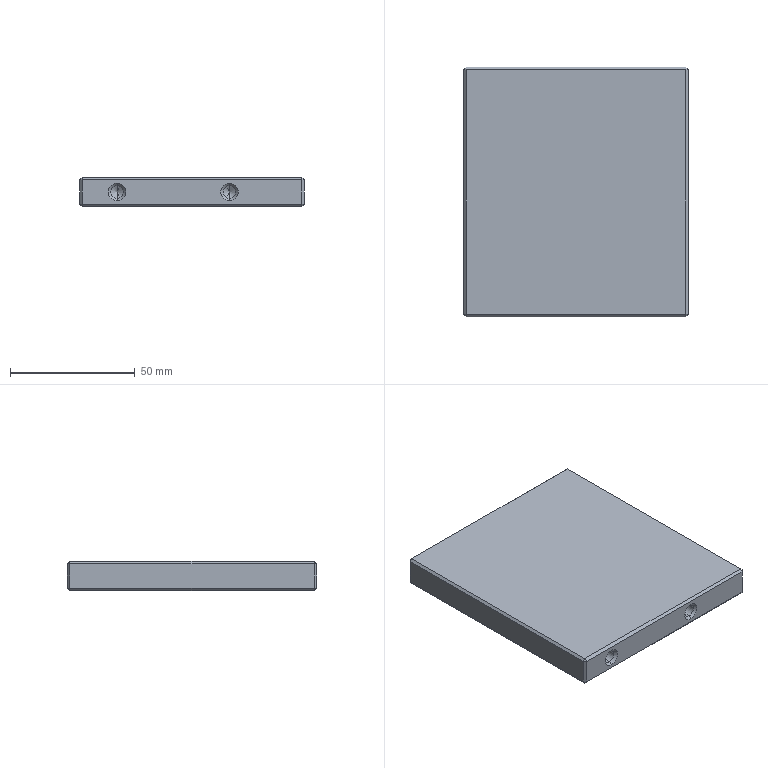Part | STEP file | 04-05 bending support plate | 1 solid | 55 faces | box 90 x 100 x 12 mm | volume 106188 mm3 | plane 27 | cone 18 | cylinder 10 | commonest cylinder face diameters 4.2 x4 5 x4 6 x2
STEP:
#1=CARTESIAN_POINT('',(0.,49.,3.));
#2=VERTEX_POINT('',#1);
#3=CARTESIAN_POINT('',(0.,49.,9.));
#4=VERTEX_POINT('',#3);
#5=CARTESIAN_POINT('',(0.,49.,6.));
#6=DIRECTION('',(0.,1.,0.));
#7=DIRECTION('',(0.,0.,-1.));
#8=AXIS2_PLACEMENT_3D('',#5,#6,#7);
#9=CIRCLE('',#8,3.);
#10=EDGE_CURVE('',#2,#4,#9,.T.);
#11=ORIENTED_EDGE('',*,*,#10,.F.);
#12=CARTESIAN_POINT('',(0.,50.,2.));
#13=VERTEX_POINT('',#12);
#14=CARTESIAN_POINT('',(0.,49.,3.));
#15=DIRECTION('',(0.,0.7071,-0.7071));
#16=VECTOR('',#15,1000.);
#17=LINE('',#14,#16);
#18=EDGE_CURVE('',#2,#13,#17,.T.);
#19=ORIENTED_EDGE('',*,*,#18,.T.);
#20=CARTESIAN_POINT('',(0.,50.,10.));
#21=VERTEX_POINT('',#20);
#22=CARTESIAN_POINT('',(0.,50.,6.));
#23=DIRECTION('',(0.,-1.,0.));
#24=DIRECTION('',(0.,0.,-1.));
#25=AXIS2_PLACEMENT_3D('',#22,#23,#24);
#26=CIRCLE('',#25,4.);
#27=EDGE_CURVE('',#21,#13,#26,.T.);
#28=ORIENTED_EDGE('',*,*,#27,.F.);
#29=CARTESIAN_POINT('',(0.,49.,9.));
#30=DIRECTION('',(0.,0.7071,0.7071));
#31=VECTOR('',#30,1000.);
#32=LINE('',#29,#31);
#33=EDGE_CURVE('',#4,#21,#32,.T.);
#34=ORIENTED_EDGE('',*,*,#33,.F.);
#35=EDGE_LOOP('',(#11,#19,#28,#34));
#36=FACE_OUTER_BOUND('',#35,.T.);
#37=CARTESIAN_POINT('',(0.,49.,6.));
#38=DIRECTION('',(0.,1.,0.));
#39=DIRECTION('',(0.,0.,1.));
#40=AXIS2_PLACEMENT_3D('',#37,#38,#39);
#41=CONICAL_SURFACE('',#40,3.,0.7854);
#42=ADVANCED_FACE('',(#36),#41,.F.);
#43=CARTESIAN_POINT('',(-30.,49.,3.9));
#44=VERTEX_POINT('',#43);
#45=CARTESIAN_POINT('',(-30.,49.,8.1));
#46=VERTEX_POINT('',#45);
#47=CARTESIAN_POINT('',(-30.,49.,6.));
#48=DIRECTION('',(0.,1.,0.));
#49=DIRECTION('',(0.,0.,-1.));
#50=AXIS2_PLACEMENT_3D('',#47,#48,#49);
#51=CIRCLE('',#50,2.1);
#52=EDGE_CURVE('',#44,#46,#51,.T.);
#53=ORIENTED_EDGE('',*,*,#52,.F.);
#54=CARTESIAN_POINT('',(-30.,50.,2.9));
#55=VERTEX_POINT('',#54);
#56=CARTESIAN_POINT('',(-30.,49.,3.9));
#57=DIRECTION('',(0.,0.7071,-0.7071));
#58=VECTOR('',#57,1000.);
#59=LINE('',#56,#58);
#60=EDGE_CURVE('',#44,#55,#59,.T.);
#61=ORIENTED_EDGE('',*,*,#60,.T.);
#62=CARTESIAN_POINT('',(-30.,50.,9.1));
#63=VERTEX_POINT('',#62);
#64=CARTESIAN_POINT('',(-30.,50.,6.));
#65=DIRECTION('',(0.,-1.,0.));
#66=DIRECTION('',(0.,0.,-1.));
#67=AXIS2_PLACEMENT_3D('',#64,#65,#66);
#68=CIRCLE('',#67,3.1);
#69=EDGE_CURVE('',#63,#55,#68,.T.);
#70=ORIENTED_EDGE('',*,*,#69,.F.);
#71=CARTESIAN_POINT('',(-30.,49.,8.1));
#72=DIRECTION('',(0.,0.7071,0.7071));
#73=VECTOR('',#72,1000.);
#74=LINE('',#71,#73);
#75=EDGE_CURVE('',#46,#63,#74,.T.);
#76=ORIENTED_EDGE('',*,*,#75,.F.);
#77=EDGE_LOOP('',(#53,#61,#70,#76));
#78=FACE_OUTER_BOUND('',#77,.T.);
#79=CARTESIAN_POINT('',(-30.,49.,6.));
#80=DIRECTION('',(0.,1.,0.));
#81=DIRECTION('',(0.,0.,1.));
#82=AXIS2_PLACEMENT_3D('',#79,#80,#81);
#83=CONICAL_SURFACE('',#82,2.1,0.7854);
#84=ADVANCED_FACE('',(#78),#83,.F.);
#85=CARTESIAN_POINT('',(30.,49.,3.9));
#86=VERTEX_POINT('',#85);
#87=CARTESIAN_POINT('',(30.,49.,8.1));
#88=VERTEX_POINT('',#87);
#89=CARTESIAN_POINT('',(30.,49.,6.));
#90=DIRECTION('',(0.,1.,0.));
#91=DIRECTION('',(0.,0.,-1.));
#92=AXIS2_PLACEMENT_3D('',#89,#90,#91);
#93=CIRCLE('',#92,2.1);
#94=EDGE_CURVE('',#86,#88,#93,.T.);
#95=ORIENTED_EDGE('',*,*,#94,.F.);
#96=CARTESIAN_POINT('',(30.,50.,2.9));
#97=VERTEX_POINT('',#96);
#98=CARTESIAN_POINT('',(30.,49.,3.9));
#99=DIRECTION('',(0.,0.7071,-0.7071));
#100=VECTOR('',#99,1000.);
#101=LINE('',#98,#100);
#102=EDGE_CURVE('',#86,#97,#101,.T.);
#103=ORIENTED_EDGE('',*,*,#102,.T.);
#104=CARTESIAN_POINT('',(30.,50.,9.1));
#105=VERTEX_POINT('',#104);
#106=CARTESIAN_POINT('',(30.,50.,6.));
#107=DIRECTION('',(0.,-1.,0.));
#108=DIRECTION('',(0.,0.,-1.));
#109=AXIS2_PLACEMENT_3D('',#106,#107,#108);
#110=CIRCLE('',#109,3.1);
#111=EDGE_CURVE('',#105,#97,#110,.T.);
#112=ORIENTED_EDGE('',*,*,#111,.F.);
#113=CARTESIAN_POINT('',(30.,49.,8.1));
#114=DIRECTION('',(0.,0.7071,0.7071));
#115=VECTOR('',#114,1000.);
#116=LINE('',#113,#115);
#117=EDGE_CURVE('',#88,#105,#116,.T.);
#118=ORIENTED_EDGE('',*,*,#117,.F.);
#119=EDGE_LOOP('',(#95,#103,#112,#118));
#120=FACE_OUTER_BOUND('',#119,.T.);
#121=CARTESIAN_POINT('',(30.,49.,6.));
#122=DIRECTION('',(0.,1.,0.));
#123=DIRECTION('',(0.,0.,1.));
#124=AXIS2_PLACEMENT_3D('',#121,#122,#123);
#125=CONICAL_SURFACE('',#124,2.1,0.7854);
#126=ADVANCED_FACE('',(#120),#125,.F.);
#127=CARTESIAN_POINT('',(-30.,-49.,8.5));
#128=VERTEX_POINT('',#127);
#129=CARTESIAN_POINT('',(-30.,-49.,3.5));
#130=VERTEX_POINT('',#129);
#131=CARTESIAN_POINT('',(-30.,-49.,6.));
#132=DIRECTION('',(0.,-1.,0.));
#133=DIRECTION('',(0.,0.,1.));
#134=AXIS2_PLACEMENT_3D('',#131,#132,#133);
#135=CIRCLE('',#134,2.5);
#136=EDGE_CURVE('',#128,#130,#135,.T.);
#137=ORIENTED_EDGE('',*,*,#136,.F.);
#138=CARTESIAN_POINT('',(-30.,-50.,9.5));
#139=VERTEX_POINT('',#138);
#140=CARTESIAN_POINT('',(-30.,-49.,8.5));
#141=DIRECTION('',(0.,-0.7071,0.7071));
#142=VECTOR('',#141,1000.);
#143=LINE('',#140,#142);
#144=EDGE_CURVE('',#128,#139,#143,.T.);
#145=ORIENTED_EDGE('',*,*,#144,.T.);
#146=CARTESIAN_POINT('',(-30.,-50.,2.5));
#147=VERTEX_POINT('',#146);
#148=CARTESIAN_POINT('',(-30.,-50.,6.));
#149=DIRECTION('',(0.,1.,0.));
#150=DIRECTION('',(0.,0.,1.));
#151=AXIS2_PLACEMENT_3D('',#148,#149,#150);
#152=CIRCLE('',#151,3.5);
#153=EDGE_CURVE('',#147,#139,#152,.T.);
#154=ORIENTED_EDGE('',*,*,#153,.F.);
#155=CARTESIAN_POINT('',(-30.,-49.,3.5));
#156=DIRECTION('',(0.,-0.7071,-0.7071));
#157=VECTOR('',#156,1000.);
#158=LINE('',#155,#157);
#159=EDGE_CURVE('',#130,#147,#158,.T.);
#160=ORIENTED_EDGE('',*,*,#159,.F.);
#161=EDGE_LOOP('',(#137,#145,#154,#160));
#162=FACE_OUTER_BOUND('',#161,.T.);
#163=CARTESIAN_POINT('',(-30.,-49.,6.));
#164=DIRECTION('',(0.,-1.,0.));
#165=DIRECTION('',(0.,0.,-1.));
#166=AXIS2_PLACEMENT_3D('',#163,#164,#165);
#167=CONICAL_SURFACE('',#166,2.5,0.7854);
#168=ADVANCED_FACE('',(#162),#167,.F.);
#169=CARTESIAN_POINT('',(15.,-49.,8.5));
#170=VERTEX_POINT('',#169);
#171=CARTESIAN_POINT('',(15.,-49.,3.5));
#172=VERTEX_POINT('',#171);
#173=CARTESIAN_POINT('',(15.,-49.,6.));
#174=DIRECTION('',(0.,-1.,0.));
#175=DIRECTION('',(0.,0.,1.));
#176=AXIS2_PLACEMENT_3D('',#173,#174,#175);
#177=CIRCLE('',#176,2.5);
#178=EDGE_CURVE('',#170,#172,#177,.T.);
#179=ORIENTED_EDGE('',*,*,#178,.F.);
#180=CARTESIAN_POINT('',(15.,-50.,9.5));
#181=VERTEX_POINT('',#180);
#182=CARTESIAN_POINT('',(15.,-49.,8.5));
#183=DIRECTION('',(0.,-0.7071,0.7071));
#184=VECTOR('',#183,1000.);
#185=LINE('',#182,#184);
#186=EDGE_CURVE('',#170,#181,#185,.T.);
#187=ORIENTED_EDGE('',*,*,#186,.T.);
#188=CARTESIAN_POINT('',(15.,-50.,2.5));
#189=VERTEX_POINT('',#188);
#190=CARTESIAN_POINT('',(15.,-50.,6.));
#191=DIRECTION('',(0.,1.,0.));
#192=DIRECTION('',(0.,0.,1.));
#193=AXIS2_PLACEMENT_3D('',#190,#191,#192);
#194=CIRCLE('',#193,3.5);
#195=EDGE_CURVE('',#189,#181,#194,.T.);
#196=ORIENTED_EDGE('',*,*,#195,.F.);
#197=CARTESIAN_POINT('',(15.,-49.,3.5));
#198=DIRECTION('',(0.,-0.7071,-0.7071));
#199=VECTOR('',#198,1000.);
#200=LINE('',#197,#199);
#201=EDGE_CURVE('',#172,#189,#200,.T.);
#202=ORIENTED_EDGE('',*,*,#201,.F.);
#203=EDGE_LOOP('',(#179,#187,#196,#202));
#204=FACE_OUTER_BOUND('',#203,.T.);
#205=CARTESIAN_POINT('',(15.,-49.,6.));
#206=DIRECTION('',(0.,-1.,0.));
#207=DIRECTION('',(0.,0.,-1.));
#208=AXIS2_PLACEMENT_3D('',#205,#206,#207);
#209=CONICAL_SURFACE('',#208,2.5,0.7854);
#210=ADVANCED_FACE('',(#204),#209,.F.);
#211=CARTESIAN_POINT('',(0.,40.,3.));
#212=VERTEX_POINT('',#211);
#213=CARTESIAN_POINT('',(0.,40.,9.));
#214=VERTEX_POINT('',#213);
#215=CARTESIAN_POINT('',(0.,40.,6.));
#216=DIRECTION('',(0.,1.,0.));
#217=DIRECTION('',(0.,0.,1.));
#218=AXIS2_PLACEMENT_3D('',#215,#216,#217);
#219=CIRCLE('',#218,3.);
#220=EDGE_CURVE('',#212,#214,#219,.T.);
#221=ORIENTED_EDGE('',*,*,#220,.F.);
#222=CARTESIAN_POINT('',(0.,40.,3.));
#223=DIRECTION('',(0.,1.,0.));
#224=VECTOR('',#223,1000.);
#225=LINE('',#222,#224);
#226=EDGE_CURVE('',#212,#2,#225,.T.);
#227=ORIENTED_EDGE('',*,*,#226,.T.);
#228=ORIENTED_EDGE('',*,*,#10,.T.);
#229=CARTESIAN_POINT('',(0.,40.,9.));
#230=DIRECTION('',(0.,1.,0.));
#231=VECTOR('',#230,1000.);
#232=LINE('',#229,#231);
#233=EDGE_CURVE('',#214,#4,#232,.T.);
#234=ORIENTED_EDGE('',*,*,#233,.F.);
#235=EDGE_LOOP('',(#221,#227,#228,#234));
#236=FACE_OUTER_BOUND('',#235,.T.);
#237=CARTESIAN_POINT('',(0.,40.,6.));
#238=DIRECTION('',(0.,1.,0.));
#239=DIRECTION('',(0.,0.,1.));
#240=AXIS2_PLACEMENT_3D('',#237,#238,#239);
#241=CYLINDRICAL_SURFACE('',#240,3.);
#242=ADVANCED_FACE('',(#236),#241,.F.);
#243=CARTESIAN_POINT('',(-30.,36.,3.9));
#244=VERTEX_POINT('',#243);
#245=CARTESIAN_POINT('',(-30.,36.,8.1));
#246=VERTEX_POINT('',#245);
#247=CARTESIAN_POINT('',(-30.,36.,6.));
#248=DIRECTION('',(0.,1.,0.));
#249=DIRECTION('',(0.,0.,1.));
#250=AXIS2_PLACEMENT_3D('',#247,#248,#249);
#251=CIRCLE('',#250,2.1);
#252=EDGE_CURVE('',#244,#246,#251,.T.);
#253=ORIENTED_EDGE('',*,*,#252,.F.);
#254=CARTESIAN_POINT('',(-30.,50.,3.9));
#255=DIRECTION('',(0.,1.,0.));
#256=VECTOR('',#255,1000.);
#257=LINE('',#254,#256);
#258=EDGE_CURVE('',#244,#44,#257,.T.);
#259=ORIENTED_EDGE('',*,*,#258,.T.);
#260=ORIENTED_EDGE('',*,*,#52,.T.);
#261=CARTESIAN_POINT('',(-30.,50.,8.1));
#262=DIRECTION('',(0.,1.,0.));
#263=VECTOR('',#262,1000.);
#264=LINE('',#261,#263);
#265=EDGE_CURVE('',#246,#46,#264,.T.);
#266=ORIENTED_EDGE('',*,*,#265,.F.);
#267=EDGE_LOOP('',(#253,#259,#260,#266));
#268=FACE_OUTER_BOUND('',#267,.T.);
#269=CARTESIAN_POINT('',(-30.,50.,6.));
#270=DIRECTION('',(0.,1.,0.));
#271=DIRECTION('',(0.,0.,1.));
#272=AXIS2_PLACEMENT_3D('',#269,#270,#271);
#273=CYLINDRICAL_SURFACE('',#272,2.1);
#274=ADVANCED_FACE('',(#268),#273,.F.);
#275=CARTESIAN_POINT('',(-30.,34.738,6.));
#276=VERTEX_POINT('',#275);
#277=CARTESIAN_POINT('',(-30.,36.,8.1));
#278=DIRECTION('',(0.,0.515,0.8572));
#279=VECTOR('',#278,1000.);
#280=LINE('',#277,#279);
#281=EDGE_CURVE('',#276,#246,#280,.T.);
#282=ORIENTED_EDGE('',*,*,#281,.F.);
#283=CARTESIAN_POINT('',(-30.,36.,3.9));
#284=DIRECTION('',(0.,0.515,-0.8572));
#285=VECTOR('',#284,1000.);
#286=LINE('',#283,#285);
#287=EDGE_CURVE('',#276,#244,#286,.T.);
#288=ORIENTED_EDGE('',*,*,#287,.T.);
#289=ORIENTED_EDGE('',*,*,#252,.T.);
#290=EDGE_LOOP('',(#282,#288,#289));
#291=FACE_OUTER_BOUND('',#290,.T.);
#292=CARTESIAN_POINT('',(-30.,36.,6.));
#293=DIRECTION('',(0.,1.,0.));
#294=DIRECTION('',(0.,0.,1.));
#295=AXIS2_PLACEMENT_3D('',#292,#293,#294);
#296=CONICAL_SURFACE('',#295,2.1,1.03);
#297=ADVANCED_FACE('',(#291),#296,.F.);
#298=CARTESIAN_POINT('',(30.,36.,3.9));
#299=VERTEX_POINT('',#298);
#300=CARTESIAN_POINT('',(30.,36.,8.1));
#301=VERTEX_POINT('',#300);
#302=CARTESIAN_POINT('',(30.,36.,6.));
#303=DIRECTION('',(0.,1.,0.));
#304=DIRECTION('',(0.,0.,1.));
#305=AXIS2_PLACEMENT_3D('',#302,#303,#304);
#306=CIRCLE('',#305,2.1);
#307=EDGE_CURVE('',#299,#301,#306,.T.);
#308=ORIENTED_EDGE('',*,*,#307,.F.);
#309=CARTESIAN_POINT('',(30.,50.,3.9));
#310=DIRECTION('',(0.,1.,0.));
#311=VECTOR('',#310,1000.);
#312=LINE('',#309,#311);
#313=EDGE_CURVE('',#299,#86,#312,.T.);
#314=ORIENTED_EDGE('',*,*,#313,.T.);
#315=ORIENTED_EDGE('',*,*,#94,.T.);
#316=CARTESIAN_POINT('',(30.,50.,8.1));
#317=DIRECTION('',(0.,1.,0.));
#318=VECTOR('',#317,1000.);
#319=LINE('',#316,#318);
#320=EDGE_CURVE('',#301,#88,#319,.T.);
#321=ORIENTED_EDGE('',*,*,#320,.F.);
#322=EDGE_LOOP('',(#308,#314,#315,#321));
#323=FACE_OUTER_BOUND('',#322,.T.);
#324=CARTESIAN_POINT('',(30.,50.,6.));
#325=DIRECTION('',(0.,1.,0.));
#326=DIRECTION('',(0.,0.,1.));
#327=AXIS2_PLACEMENT_3D('',#324,#325,#326);
#328=CYLINDRICAL_SURFACE('',#327,2.1);
#329=ADVANCED_FACE('',(#323),#328,.F.);
#330=CARTESIAN_POINT('',(30.,34.738,6.));
#331=VERTEX_POINT('',#330);
#332=CARTESIAN_POINT('',(30.,36.,8.1));
#333=DIRECTION('',(0.,0.515,0.8572));
#334=VECTOR('',#333,1000.);
#335=LINE('',#332,#334);
#336=EDGE_CURVE('',#331,#301,#335,.T.);
#337=ORIENTED_EDGE('',*,*,#336,.F.);
#338=CARTESIAN_POINT('',(30.,36.,3.9));
#339=DIRECTION('',(0.,0.515,-0.8572));
#340=VECTOR('',#339,1000.);
#341=LINE('',#338,#340);
#342=EDGE_CURVE('',#331,#299,#341,.T.);
#343=ORIENTED_EDGE('',*,*,#342,.T.);
#344=ORIENTED_EDGE('',*,*,#307,.T.);
#345=EDGE_LOOP('',(#337,#343,#344));
#346=FACE_OUTER_BOUND('',#345,.T.);
#347=CARTESIAN_POINT('',(30.,36.,6.));
#348=DIRECTION('',(0.,1.,0.));
#349=DIRECTION('',(0.,0.,1.));
#350=AXIS2_PLACEMENT_3D('',#347,#348,#349);
#351=CONICAL_SURFACE('',#350,2.1,1.03);
#352=ADVANCED_FACE('',(#346),#351,.F.);
#353=CARTESIAN_POINT('',(-30.,-33.,8.5));
#354=VERTEX_POINT('',#353);
#355=CARTESIAN_POINT('',(-30.,-33.,3.5));
#356=VERTEX_POINT('',#355);
#357=CARTESIAN_POINT('',(-30.,-33.,6.));
#358=DIRECTION('',(0.,-1.,0.));
#359=DIRECTION('',(0.,0.,-1.));
#360=AXIS2_PLACEMENT_3D('',#357,#358,#359);
#361=CIRCLE('',#360,2.5);
#362=EDGE_CURVE('',#354,#356,#361,.T.);
#363=ORIENTED_EDGE('',*,*,#362,.F.);
#364=CARTESIAN_POINT('',(-30.,-50.,8.5));
#365=DIRECTION('',(0.,-1.,0.));
#366=VECTOR('',#365,1000.);
#367=LINE('',#364,#366);
#368=EDGE_CURVE('',#354,#128,#367,.T.);
#369=ORIENTED_EDGE('',*,*,#368,.T.);
#370=ORIENTED_EDGE('',*,*,#136,.T.);
#371=CARTESIAN_POINT('',(-30.,-50.,3.5));
#372=DIRECTION('',(0.,-1.,0.));
#373=VECTOR('',#372,1000.);
#374=LINE('',#371,#373);
#375=EDGE_CURVE('',#356,#130,#374,.T.);
#376=ORIENTED_EDGE('',*,*,#375,.F.);
#377=EDGE_LOOP('',(#363,#369,#370,#376));
#378=FACE_OUTER_BOUND('',#377,.T.);
#379=CARTESIAN_POINT('',(-30.,-50.,6.));
#380=DIRECTION('',(0.,-1.,0.));
#381=DIRECTION('',(0.,0.,-1.));
#382=AXIS2_PLACEMENT_3D('',#379,#380,#381);
#383=CYLINDRICAL_SURFACE('',#382,2.5);
#384=ADVANCED_FACE('',(#378),#383,.F.);
#385=CARTESIAN_POINT('',(-30.,-31.498,6.));
#386=VERTEX_POINT('',#385);
#387=CARTESIAN_POINT('',(-30.,-33.,3.5));
#388=DIRECTION('',(0.,-0.515,-0.8572));
#389=VECTOR('',#388,1000.);
#390=LINE('',#387,#389);
#391=EDGE_CURVE('',#386,#356,#390,.T.);
#392=ORIENTED_EDGE('',*,*,#391,.F.);
#393=CARTESIAN_POINT('',(-30.,-33.,8.5));
#394=DIRECTION('',(0.,-0.515,0.8572));
#395=VECTOR('',#394,1000.);
#396=LINE('',#393,#395);
#397=EDGE_CURVE('',#386,#354,#396,.T.);
#398=ORIENTED_EDGE('',*,*,#397,.T.);
#399=ORIENTED_EDGE('',*,*,#362,.T.);
#400=EDGE_LOOP('',(#392,#398,#399));
#401=FACE_OUTER_BOUND('',#400,.T.);
#402=CARTESIAN_POINT('',(-30.,-33.,6.));
#403=DIRECTION('',(0.,-1.,0.));
#404=DIRECTION('',(0.,0.,-1.));
#405=AXIS2_PLACEMENT_3D('',#402,#403,#404);
#406=CONICAL_SURFACE('',#405,2.5,1.03);
#407=ADVANCED_FACE('',(#401),#406,.F.);
#408=CARTESIAN_POINT('',(15.,-33.,8.5));
#409=VERTEX_POINT('',#408);
#410=CARTESIAN_POINT('',(15.,-33.,3.5));
#411=VERTEX_POINT('',#410);
#412=CARTESIAN_POINT('',(15.,-33.,6.));
#413=DIRECTION('',(0.,-1.,0.));
#414=DIRECTION('',(0.,0.,-1.));
#415=AXIS2_PLACEMENT_3D('',#412,#413,#414);
#416=CIRCLE('',#415,2.5);
#417=EDGE_CURVE('',#409,#411,#416,.T.);
#418=ORIENTED_EDGE('',*,*,#417,.F.);
#419=CARTESIAN_POINT('',(15.,-50.,8.5));
#420=DIRECTION('',(0.,-1.,0.));
#421=VECTOR('',#420,1000.);
#422=LINE('',#419,#421);
#423=EDGE_CURVE('',#409,#170,#422,.T.);
#424=ORIENTED_EDGE('',*,*,#423,.T.);
#425=ORIENTED_EDGE('',*,*,#178,.T.);
#426=CARTESIAN_POINT('',(15.,-50.,3.5));
#427=DIRECTION('',(0.,-1.,0.));
#428=VECTOR('',#427,1000.);
#429=LINE('',#426,#428);
#430=EDGE_CURVE('',#411,#172,#429,.T.);
#431=ORIENTED_EDGE('',*,*,#430,.F.);
#432=EDGE_LOOP('',(#418,#424,#425,#431));
#433=FACE_OUTER_BOUND('',#432,.T.);
#434=CARTESIAN_POINT('',(15.,-50.,6.));
#435=DIRECTION('',(0.,-1.,0.));
#436=DIRECTION('',(0.,0.,-1.));
#437=AXIS2_PLACEMENT_3D('',#434,#435,#436);
#438=CYLINDRICAL_SURFACE('',#437,2.5);
#439=ADVANCED_FACE('',(#433),#438,.F.);
#440=CARTESIAN_POINT('',(15.,-31.498,6.));
#441=VERTEX_POINT('',#440);
#442=CARTESIAN_POINT('',(15.,-33.,3.5));
#443=DIRECTION('',(0.,-0.515,-0.8572));
#444=VECTOR('',#443,1000.);
#445=LINE('',#442,#444);
#446=EDGE_CURVE('',#441,#411,#445,.T.);
#447=ORIENTED_EDGE('',*,*,#446,.F.);
#448=CARTESIAN_POINT('',(15.,-33.,8.5));
#449=DIRECTION('',(0.,-0.515,0.8572));
#450=VECTOR('',#449,1000.);
#451=LINE('',#448,#450);
#452=EDGE_CURVE('',#441,#409,#451,.T.);
#453=ORIENTED_EDGE('',*,*,#452,.T.);
#454=ORIENTED_EDGE('',*,*,#417,.T.);
#455=EDGE_LOOP('',(#447,#453,#454));
#456=FACE_OUTER_BOUND('',#455,.T.);
#457=CARTESIAN_POINT('',(15.,-33.,6.));
#458=DIRECTION('',(0.,-1.,0.));
#459=DIRECTION('',(0.,0.,-1.));
#460=AXIS2_PLACEMENT_3D('',#457,#458,#459);
#461=CONICAL_SURFACE('',#460,2.5,1.03);
#462=ADVANCED_FACE('',(#456),#461,.F.);
#463=CARTESIAN_POINT('',(45.,-49.,11.));
#464=VERTEX_POINT('',#463);
#465=CARTESIAN_POINT('',(45.,-49.,1.));
#466=VERTEX_POINT('',#465);
#467=CARTESIAN_POINT('',(45.,-49.,12.));
#468=DIRECTION('',(0.,0.,-1.));
#469=VECTOR('',#468,1000.);
#470=LINE('',#467,#469);
#471=EDGE_CURVE('',#464,#466,#470,.T.);
#472=ORIENTED_EDGE('',*,*,#471,.T.);
#473=CARTESIAN_POINT('',(45.,49.,1.));
#474=VERTEX_POINT('',#473);
#475=CARTESIAN_POINT('',(45.,50.,1.));
#476=DIRECTION('',(0.,1.,0.));
#477=VECTOR('',#476,1000.);
#478=LINE('',#475,#477);
#479=EDGE_CURVE('',#466,#474,#478,.T.);
#480=ORIENTED_EDGE('',*,*,#479,.T.);
#481=CARTESIAN_POINT('',(45.,49.,11.));
#482=VERTEX_POINT('',#481);
#483=CARTESIAN_POINT('',(45.,49.,12.));
#484=DIRECTION('',(0.,0.,1.));
#485=VECTOR('',#484,1000.);
#486=LINE('',#483,#485);
#487=EDGE_CURVE('',#474,#482,#486,.T.);
#488=ORIENTED_EDGE('',*,*,#487,.T.);
#489=CARTESIAN_POINT('',(45.,-50.,11.));
#490=DIRECTION('',(0.,-1.,0.));
#491=VECTOR('',#490,1000.);
#492=LINE('',#489,#491);
#493=EDGE_CURVE('',#482,#464,#492,.T.);
#494=ORIENTED_EDGE('',*,*,#493,.T.);
#495=EDGE_LOOP('',(#472,#480,#488,#494));
#496=FACE_OUTER_BOUND('',#495,.T.);
#497=CARTESIAN_POINT('',(45.,50.,12.));
#498=DIRECTION('',(-1.,0.,0.));
#499=DIRECTION('',(0.,-1.,0.));
#500=AXIS2_PLACEMENT_3D('',#497,#498,#499);
#501=PLANE('',#500);
#502=ADVANCED_FACE('',(#496),#501,.F.);
#503=ORIENTED_EDGE('',*,*,#111,.T.);
#504=CARTESIAN_POINT('',(30.,50.,6.));
#505=DIRECTION('',(0.,-1.,0.));
#506=DIRECTION('',(0.,0.,-1.));
#507=AXIS2_PLACEMENT_3D('',#504,#505,#506);
#508=CIRCLE('',#507,3.1);
#509=EDGE_CURVE('',#97,#105,#508,.T.);
#510=ORIENTED_EDGE('',*,*,#509,.T.);
#511=EDGE_LOOP('',(#503,#510));
#512=FACE_BOUND('',#511,.T.);
#513=ORIENTED_EDGE('',*,*,#69,.T.);
#514=CARTESIAN_POINT('',(-30.,50.,6.));
#515=DIRECTION('',(0.,-1.,0.));
#516=DIRECTION('',(0.,0.,-1.));
#517=AXIS2_PLACEMENT_3D('',#514,#515,#516);
#518=CIRCLE('',#517,3.1);
#519=EDGE_CURVE('',#55,#63,#518,.T.);
#520=ORIENTED_EDGE('',*,*,#519,.T.);
#521=EDGE_LOOP('',(#513,#520));
#522=FACE_BOUND('',#521,.T.);
#523=ORIENTED_EDGE('',*,*,#27,.T.);
#524=CARTESIAN_POINT('',(0.,50.,6.));
#525=DIRECTION('',(0.,-1.,0.));
#526=DIRECTION('',(0.,0.,-1.));
#527=AXIS2_PLACEMENT_3D('',#524,#525,#526);
#528=CIRCLE('',#527,4.);
#529=EDGE_CURVE('',#13,#21,#528,.T.);
#530=ORIENTED_EDGE('',*,*,#529,.T.);
#531=EDGE_LOOP('',(#523,#530));
#532=FACE_BOUND('',#531,.T.);
#533=CARTESIAN_POINT('',(44.,50.,11.));
#534=VERTEX_POINT('',#533);
#535=CARTESIAN_POINT('',(44.,50.,1.));
#536=VERTEX_POINT('',#535);
#537=CARTESIAN_POINT('',(44.,50.,12.));
#538=DIRECTION('',(0.,0.,-1.));
#539=VECTOR('',#538,1000.);
#540=LINE('',#537,#539);
#541=EDGE_CURVE('',#534,#536,#540,.T.);
#542=ORIENTED_EDGE('',*,*,#541,.T.);
#543=CARTESIAN_POINT('',(-44.,50.,1.));
#544=VERTEX_POINT('',#543);
#545=CARTESIAN_POINT('',(-45.,50.,1.));
#546=DIRECTION('',(-1.,0.,0.));
#547=VECTOR('',#546,1000.);
#548=LINE('',#545,#547);
#549=EDGE_CURVE('',#536,#544,#548,.T.);
#550=ORIENTED_EDGE('',*,*,#549,.T.);
#551=CARTESIAN_POINT('',(-44.,50.,11.));
#552=VERTEX_POINT('',#551);
#553=CARTESIAN_POINT('',(-44.,50.,12.));
#554=DIRECTION('',(0.,0.,1.));
#555=VECTOR('',#554,1000.);
#556=LINE('',#553,#555);
#557=EDGE_CURVE('',#544,#552,#556,.T.);
#558=ORIENTED_EDGE('',*,*,#557,.T.);
#559=CARTESIAN_POINT('',(45.,50.,11.));
#560=DIRECTION('',(1.,0.,0.));
#561=VECTOR('',#560,1000.);
#562=LINE('',#559,#561);
#563=EDGE_CURVE('',#552,#534,#562,.T.);
#564=ORIENTED_EDGE('',*,*,#563,.T.);
#565=EDGE_LOOP('',(#542,#550,#558,#564));
#566=FACE_OUTER_BOUND('',#565,.T.);
#567=CARTESIAN_POINT('',(-45.,50.,12.));
#568=DIRECTION('',(0.,-1.,0.));
#569=DIRECTION('',(0.,0.,-1.));
#570=AXIS2_PLACEMENT_3D('',#567,#568,#569);
#571=PLANE('',#570);
#572=ADVANCED_FACE('',(#512,#522,#532,#566),#571,.F.);
#573=CARTESIAN_POINT('',(-45.,-49.,11.));
#574=VERTEX_POINT('',#573);
#575=CARTESIAN_POINT('',(-45.,49.,11.));
#576=VERTEX_POINT('',#575);
#577=CARTESIAN_POINT('',(-45.,50.,11.));
#578=DIRECTION('',(0.,1.,0.));
#579=VECTOR('',#578,1000.);
#580=LINE('',#577,#579);
#581=EDGE_CURVE('',#574,#576,#580,.T.);
#582=ORIENTED_EDGE('',*,*,#581,.T.);
#583=CARTESIAN_POINT('',(-45.,49.,1.));
#584=VERTEX_POINT('',#583);
#585=CARTESIAN_POINT('',(-45.,49.,12.));
#586=DIRECTION('',(0.,0.,-1.));
#587=VECTOR('',#586,1000.);
#588=LINE('',#585,#587);
#589=EDGE_CURVE('',#576,#584,#588,.T.);
#590=ORIENTED_EDGE('',*,*,#589,.T.);
#591=CARTESIAN_POINT('',(-45.,-49.,1.));
#592=VERTEX_POINT('',#591);
#593=CARTESIAN_POINT('',(-45.,50.,1.));
#594=DIRECTION('',(0.,-1.,0.));
#595=VECTOR('',#594,1000.);
#596=LINE('',#593,#595);
#597=EDGE_CURVE('',#584,#592,#596,.T.);
#598=ORIENTED_EDGE('',*,*,#597,.T.);
#599=CARTESIAN_POINT('',(-45.,-49.,12.));
#600=DIRECTION('',(0.,0.,1.));
#601=VECTOR('',#600,1000.);
#602=LINE('',#599,#601);
#603=EDGE_CURVE('',#592,#574,#602,.T.);
#604=ORIENTED_EDGE('',*,*,#603,.T.);
#605=EDGE_LOOP('',(#582,#590,#598,#604));
#606=FACE_OUTER_BOUND('',#605,.T.);
#607=CARTESIAN_POINT('',(-45.,50.,12.));
#608=DIRECTION('',(1.,0.,0.));
#609=DIRECTION('',(0.,1.,0.));
#610=AXIS2_PLACEMENT_3D('',#607,#608,#609);
#611=PLANE('',#610);
#612=ADVANCED_FACE('',(#606),#611,.F.);
#613=ORIENTED_EDGE('',*,*,#195,.T.);
#614=CARTESIAN_POINT('',(15.,-50.,6.));
#615=DIRECTION('',(0.,1.,0.));
#616=DIRECTION('',(0.,0.,1.));
#617=AXIS2_PLACEMENT_3D('',#614,#615,#616);
#618=CIRCLE('',#617,3.5);
#619=EDGE_CURVE('',#181,#189,#618,.T.);
#620=ORIENTED_EDGE('',*,*,#619,.T.);
#621=EDGE_LOOP('',(#613,#620));
#622=FACE_BOUND('',#621,.T.);
#623=ORIENTED_EDGE('',*,*,#153,.T.);
#624=CARTESIAN_POINT('',(-30.,-50.,6.));
#625=DIRECTION('',(0.,1.,0.));
#626=DIRECTION('',(0.,0.,1.));
#627=AXIS2_PLACEMENT_3D('',#624,#625,#626);
#628=CIRCLE('',#627,3.5);
#629=EDGE_CURVE('',#139,#147,#628,.T.);
#630=ORIENTED_EDGE('',*,*,#629,.T.);
#631=EDGE_LOOP('',(#623,#630));
#632=FACE_BOUND('',#631,.T.);
#633=CARTESIAN_POINT('',(-44.,-50.,1.));
#634=VERTEX_POINT('',#633);
#635=CARTESIAN_POINT('',(44.,-50.,1.));
#636=VERTEX_POINT('',#635);
#637=CARTESIAN_POINT('',(-45.,-50.,1.));
#638=DIRECTION('',(1.,0.,0.));
#639=VECTOR('',#638,1000.);
#640=LINE('',#637,#639);
#641=EDGE_CURVE('',#634,#636,#640,.T.);
#642=ORIENTED_EDGE('',*,*,#641,.T.);
#643=CARTESIAN_POINT('',(44.,-50.,11.));
#644=VERTEX_POINT('',#643);
#645=CARTESIAN_POINT('',(44.,-50.,12.));
#646=DIRECTION('',(0.,0.,1.));
#647=VECTOR('',#646,1000.);
#648=LINE('',#645,#647);
#649=EDGE_CURVE('',#636,#644,#648,.T.);
#650=ORIENTED_EDGE('',*,*,#649,.T.);
#651=CARTESIAN_POINT('',(-44.,-50.,11.));
#652=VERTEX_POINT('',#651);
#653=CARTESIAN_POINT('',(-45.,-50.,11.));
#654=DIRECTION('',(-1.,0.,0.));
#655=VECTOR('',#654,1000.);
#656=LINE('',#653,#655);
#657=EDGE_CURVE('',#644,#652,#656,.T.);
#658=ORIENTED_EDGE('',*,*,#657,.T.);
#659=CARTESIAN_POINT('',(-44.,-50.,12.));
#660=DIRECTION('',(0.,0.,-1.));
#661=VECTOR('',#660,1000.);
#662=LINE('',#659,#661);
#663=EDGE_CURVE('',#652,#634,#662,.T.);
#664=ORIENTED_EDGE('',*,*,#663,.T.);
#665=EDGE_LOOP('',(#642,#650,#658,#664));
#666=FACE_OUTER_BOUND('',#665,.T.);
#667=CARTESIAN_POINT('',(-45.,-50.,12.));
#668=DIRECTION('',(0.,1.,0.));
#669=DIRECTION('',(0.,0.,1.));
#670=AXIS2_PLACEMENT_3D('',#667,#668,#669);
#671=PLANE('',#670);
#672=ADVANCED_FACE('',(#622,#632,#666),#671,.F.);
#673=CARTESIAN_POINT('',(-44.,49.,12.));
#674=VERTEX_POINT('',#673);
#675=CARTESIAN_POINT('',(-44.,-49.,12.));
#676=VERTEX_POINT('',#675);
#677=CARTESIAN_POINT('',(-44.,-50.,12.));
#678=DIRECTION('',(0.,-1.,0.));
#679=VECTOR('',#678,1000.);
#680=LINE('',#677,#679);
#681=EDGE_CURVE('',#674,#676,#680,.T.);
#682=ORIENTED_EDGE('',*,*,#681,.T.);
#683=CARTESIAN_POINT('',(44.,-49.,12.));
#684=VERTEX_POINT('',#683);
#685=CARTESIAN_POINT('',(45.,-49.,12.));
#686=DIRECTION('',(1.,0.,0.));
#687=VECTOR('',#686,1000.);
#688=LINE('',#685,#687);
#689=EDGE_CURVE('',#676,#684,#688,.T.);
#690=ORIENTED_EDGE('',*,*,#689,.T.);
#691=CARTESIAN_POINT('',(44.,49.,12.));
#692=VERTEX_POINT('',#691);
#693=CARTESIAN_POINT('',(44.,50.,12.));
#694=DIRECTION('',(0.,1.,0.));
#695=VECTOR('',#694,1000.);
#696=LINE('',#693,#695);
#697=EDGE_CURVE('',#684,#692,#696,.T.);
#698=ORIENTED_EDGE('',*,*,#697,.T.);
#699=CARTESIAN_POINT('',(-45.,49.,12.));
#700=DIRECTION('',(-1.,0.,0.));
#701=VECTOR('',#700,1000.);
#702=LINE('',#699,#701);
#703=EDGE_CURVE('',#692,#674,#702,.T.);
#704=ORIENTED_EDGE('',*,*,#703,.T.);
#705=EDGE_LOOP('',(#682,#690,#698,#704));
#706=FACE_OUTER_BOUND('',#705,.T.);
#707=CARTESIAN_POINT('',(45.,-50.,12.));
#708=DIRECTION('',(0.,0.,1.));
#709=DIRECTION('',(1.,0.,0.));
#710=AXIS2_PLACEMENT_3D('',#707,#708,#709);
#711=PLANE('',#710);
#712=ADVANCED_FACE('',(#706),#711,.T.);
#713=CARTESIAN_POINT('',(-44.,-49.,0.));
#714=VERTEX_POINT('',#713);
#715=CARTESIAN_POINT('',(-44.,49.,0.));
#716=VERTEX_POINT('',#715);
#717=CARTESIAN_POINT('',(-44.,-50.,0.));
#718=DIRECTION('',(0.,1.,0.));
#719=VECTOR('',#718,1000.);
#720=LINE('',#717,#719);
#721=EDGE_CURVE('',#714,#716,#720,.T.);
#722=ORIENTED_EDGE('',*,*,#721,.T.);
#723=CARTESIAN_POINT('',(44.,49.,0.));
#724=VERTEX_POINT('',#723);
#725=CARTESIAN_POINT('',(45.,49.,0.));
#726=DIRECTION('',(1.,0.,0.));
#727=VECTOR('',#726,1000.);
#728=LINE('',#725,#727);
#729=EDGE_CURVE('',#716,#724,#728,.T.);
#730=ORIENTED_EDGE('',*,*,#729,.T.);
#731=CARTESIAN_POINT('',(44.,-49.,0.));
#732=VERTEX_POINT('',#731);
#733=CARTESIAN_POINT('',(44.,-50.,0.));
#734=DIRECTION('',(0.,-1.,0.));
#735=VECTOR('',#734,1000.);
#736=LINE('',#733,#735);
#737=EDGE_CURVE('',#724,#732,#736,.T.);
#738=ORIENTED_EDGE('',*,*,#737,.T.);
#739=CARTESIAN_POINT('',(45.,-49.,0.));
#740=DIRECTION('',(-1.,0.,0.));
#741=VECTOR('',#740,1000.);
#742=LINE('',#739,#741);
#743=EDGE_CURVE('',#732,#714,#742,.T.);
#744=ORIENTED_EDGE('',*,*,#743,.T.);
#745=EDGE_LOOP('',(#722,#730,#738,#744));
#746=FACE_OUTER_BOUND('',#745,.T.);
#747=CARTESIAN_POINT('',(45.,-50.,0.));
#748=DIRECTION('',(0.,0.,1.));
#749=DIRECTION('',(1.,0.,0.));
#750=AXIS2_PLACEMENT_3D('',#747,#748,#749);
#751=PLANE('',#750);
#752=ADVANCED_FACE('',(#746),#751,.F.);
#753=ORIENTED_EDGE('',*,*,#452,.F.);
#754=ORIENTED_EDGE('',*,*,#446,.T.);
#755=CARTESIAN_POINT('',(15.,-33.,6.));
#756=DIRECTION('',(0.,-1.,0.));
#757=DIRECTION('',(0.,0.,-1.));
#758=AXIS2_PLACEMENT_3D('',#755,#756,#757);
#759=CIRCLE('',#758,2.5);
#760=EDGE_CURVE('',#411,#409,#759,.T.);
#761=ORIENTED_EDGE('',*,*,#760,.T.);
#762=EDGE_LOOP('',(#753,#754,#761));
#763=FACE_OUTER_BOUND('',#762,.T.);
#764=CARTESIAN_POINT('',(15.,-33.,6.));
#765=DIRECTION('',(0.,-1.,0.));
#766=DIRECTION('',(0.,0.,-1.));
#767=AXIS2_PLACEMENT_3D('',#764,#765,#766);
#768=CONICAL_SURFACE('',#767,2.5,1.03);
#769=ADVANCED_FACE('',(#763),#768,.F.);
#770=ORIENTED_EDGE('',*,*,#423,.F.);
#771=ORIENTED_EDGE('',*,*,#760,.F.);
#772=ORIENTED_EDGE('',*,*,#430,.T.);
#773=CARTESIAN_POINT('',(15.,-49.,6.));
#774=DIRECTION('',(0.,-1.,0.));
#775=DIRECTION('',(0.,0.,1.));
#776=AXIS2_PLACEMENT_3D('',#773,#774,#775);
#777=CIRCLE('',#776,2.5);
#778=EDGE_CURVE('',#172,#170,#777,.T.);
#779=ORIENTED_EDGE('',*,*,#778,.T.);
#780=EDGE_LOOP('',(#770,#771,#772,#779));
#781=FACE_OUTER_BOUND('',#780,.T.);
#782=CARTESIAN_POINT('',(15.,-50.,6.));
#783=DIRECTION('',(0.,-1.,0.));
#784=DIRECTION('',(0.,0.,-1.));
#785=AXIS2_PLACEMENT_3D('',#782,#783,#784);
#786=CYLINDRICAL_SURFACE('',#785,2.5);
#787=ADVANCED_FACE('',(#781),#786,.F.);
#788=ORIENTED_EDGE('',*,*,#397,.F.);
#789=ORIENTED_EDGE('',*,*,#391,.T.);
#790=CARTESIAN_POINT('',(-30.,-33.,6.));
#791=DIRECTION('',(0.,-1.,0.));
#792=DIRECTION('',(0.,0.,-1.));
#793=AXIS2_PLACEMENT_3D('',#790,#791,#792);
#794=CIRCLE('',#793,2.5);
#795=EDGE_CURVE('',#356,#354,#794,.T.);
#796=ORIENTED_EDGE('',*,*,#795,.T.);
#797=EDGE_LOOP('',(#788,#789,#796));
#798=FACE_OUTER_BOUND('',#797,.T.);
#799=CARTESIAN_POINT('',(-30.,-33.,6.));
#800=DIRECTION('',(0.,-1.,0.));
#801=DIRECTION('',(0.,0.,-1.));
#802=AXIS2_PLACEMENT_3D('',#799,#800,#801);
#803=CONICAL_SURFACE('',#802,2.5,1.03);
#804=ADVANCED_FACE('',(#798),#803,.F.);
#805=ORIENTED_EDGE('',*,*,#368,.F.);
#806=ORIENTED_EDGE('',*,*,#795,.F.);
#807=ORIENTED_EDGE('',*,*,#375,.T.);
#808=CARTESIAN_POINT('',(-30.,-49.,6.));
#809=DIRECTION('',(0.,-1.,0.));
#810=DIRECTION('',(0.,0.,1.));
#811=AXIS2_PLACEMENT_3D('',#808,#809,#810);
#812=CIRCLE('',#811,2.5);
#813=EDGE_CURVE('',#130,#128,#812,.T.);
#814=ORIENTED_EDGE('',*,*,#813,.T.);
#815=EDGE_LOOP('',(#805,#806,#807,#814));
#816=FACE_OUTER_BOUND('',#815,.T.);
#817=CARTESIAN_POINT('',(-30.,-50.,6.));
#818=DIRECTION('',(0.,-1.,0.));
#819=DIRECTION('',(0.,0.,-1.));
#820=AXIS2_PLACEMENT_3D('',#817,#818,#819);
#821=CYLINDRICAL_SURFACE('',#820,2.5);
#822=ADVANCED_FACE('',(#816),#821,.F.);
#823=ORIENTED_EDGE('',*,*,#342,.F.);
#824=ORIENTED_EDGE('',*,*,#336,.T.);
#825=CARTESIAN_POINT('',(30.,36.,6.));
#826=DIRECTION('',(0.,1.,0.));
#827=DIRECTION('',(0.,0.,1.));
#828=AXIS2_PLACEMENT_3D('',#825,#826,#827);
#829=CIRCLE('',#828,2.1);
#830=EDGE_CURVE('',#301,#299,#829,.T.);
#831=ORIENTED_EDGE('',*,*,#830,.T.);
#832=EDGE_LOOP('',(#823,#824,#831));
#833=FACE_OUTER_BOUND('',#832,.T.);
#834=CARTESIAN_POINT('',(30.,36.,6.));
#835=DIRECTION('',(0.,1.,0.));
#836=DIRECTION('',(0.,0.,1.));
#837=AXIS2_PLACEMENT_3D('',#834,#835,#836);
#838=CONICAL_SURFACE('',#837,2.1,1.03);
#839=ADVANCED_FACE('',(#833),#838,.F.);
#840=ORIENTED_EDGE('',*,*,#313,.F.);
#841=ORIENTED_EDGE('',*,*,#830,.F.);
#842=ORIENTED_EDGE('',*,*,#320,.T.);
#843=CARTESIAN_POINT('',(30.,49.,6.));
#844=DIRECTION('',(0.,1.,0.));
#845=DIRECTION('',(0.,0.,-1.));
#846=AXIS2_PLACEMENT_3D('',#843,#844,#845);
#847=CIRCLE('',#846,2.1);
#848=EDGE_CURVE('',#88,#86,#847,.T.);
#849=ORIENTED_EDGE('',*,*,#848,.T.);
#850=EDGE_LOOP('',(#840,#841,#842,#849));
#851=FACE_OUTER_BOUND('',#850,.T.);
#852=CARTESIAN_POINT('',(30.,50.,6.));
#853=DIRECTION('',(0.,1.,0.));
#854=DIRECTION('',(0.,0.,1.));
#855=AXIS2_PLACEMENT_3D('',#852,#853,#854);
#856=CYLINDRICAL_SURFACE('',#855,2.1);
#857=ADVANCED_FACE('',(#851),#856,.F.);
#858=ORIENTED_EDGE('',*,*,#287,.F.);
#859=ORIENTED_EDGE('',*,*,#281,.T.);
#860=CARTESIAN_POINT('',(-30.,36.,6.));
#861=DIRECTION('',(0.,1.,0.));
#862=DIRECTION('',(0.,0.,1.));
#863=AXIS2_PLACEMENT_3D('',#860,#861,#862);
#864=CIRCLE('',#863,2.1);
#865=EDGE_CURVE('',#246,#244,#864,.T.);
#866=ORIENTED_EDGE('',*,*,#865,.T.);
#867=EDGE_LOOP('',(#858,#859,#866));
#868=FACE_OUTER_BOUND('',#867,.T.);
#869=CARTESIAN_POINT('',(-30.,36.,6.));
#870=DIRECTION('',(0.,1.,0.));
#871=DIRECTION('',(0.,0.,1.));
#872=AXIS2_PLACEMENT_3D('',#869,#870,#871);
#873=CONICAL_SURFACE('',#872,2.1,1.03);
#874=ADVANCED_FACE('',(#868),#873,.F.);
#875=ORIENTED_EDGE('',*,*,#258,.F.);
#876=ORIENTED_EDGE('',*,*,#865,.F.);
#877=ORIENTED_EDGE('',*,*,#265,.T.);
#878=CARTESIAN_POINT('',(-30.,49.,6.));
#879=DIRECTION('',(0.,1.,0.));
#880=DIRECTION('',(0.,0.,-1.));
#881=AXIS2_PLACEMENT_3D('',#878,#879,#880);
#882=CIRCLE('',#881,2.1);
#883=EDGE_CURVE('',#46,#44,#882,.T.);
#884=ORIENTED_EDGE('',*,*,#883,.T.);
#885=EDGE_LOOP('',(#875,#876,#877,#884));
#886=FACE_OUTER_BOUND('',#885,.T.);
#887=CARTESIAN_POINT('',(-30.,50.,6.));
#888=DIRECTION('',(0.,1.,0.));
#889=DIRECTION('',(0.,0.,1.));
#890=AXIS2_PLACEMENT_3D('',#887,#888,#889);
#891=CYLINDRICAL_SURFACE('',#890,2.1);
#892=ADVANCED_FACE('',(#886),#891,.F.);
#893=ORIENTED_EDGE('',*,*,#226,.F.);
#894=CARTESIAN_POINT('',(0.,40.,6.));
#895=DIRECTION('',(0.,1.,0.));
#896=DIRECTION('',(0.,0.,1.));
#897=AXIS2_PLACEMENT_3D('',#894,#895,#896);
#898=CIRCLE('',#897,3.);
#899=EDGE_CURVE('',#214,#212,#898,.T.);
#900=ORIENTED_EDGE('',*,*,#899,.F.);
#901=ORIENTED_EDGE('',*,*,#233,.T.);
#902=CARTESIAN_POINT('',(0.,49.,6.));
#903=DIRECTION('',(0.,1.,0.));
#904=DIRECTION('',(0.,0.,-1.));
#905=AXIS2_PLACEMENT_3D('',#902,#903,#904);
#906=CIRCLE('',#905,3.);
#907=EDGE_CURVE('',#4,#2,#906,.T.);
#908=ORIENTED_EDGE('',*,*,#907,.T.);
#909=EDGE_LOOP('',(#893,#900,#901,#908));
#910=FACE_OUTER_BOUND('',#909,.T.);
#911=CARTESIAN_POINT('',(0.,40.,6.));
#912=DIRECTION('',(0.,1.,0.));
#913=DIRECTION('',(0.,0.,1.));
#914=AXIS2_PLACEMENT_3D('',#911,#912,#913);
#915=CYLINDRICAL_SURFACE('',#914,3.);
#916=ADVANCED_FACE('',(#910),#915,.F.);
#917=ORIENTED_EDGE('',*,*,#899,.T.);
#918=ORIENTED_EDGE('',*,*,#220,.T.);
#919=EDGE_LOOP('',(#917,#918));
#920=FACE_OUTER_BOUND('',#919,.T.);
#921=CARTESIAN_POINT('',(0.,40.,6.));
#922=DIRECTION('',(0.,1.,0.));
#923=DIRECTION('',(0.,0.,1.));
#924=AXIS2_PLACEMENT_3D('',#921,#922,#923);
#925=PLANE('',#924);
#926=ADVANCED_FACE('',(#920),#925,.T.);
#927=ORIENTED_EDGE('',*,*,#186,.F.);
#928=ORIENTED_EDGE('',*,*,#778,.F.);
#929=ORIENTED_EDGE('',*,*,#201,.T.);
#930=ORIENTED_EDGE('',*,*,#619,.F.);
#931=EDGE_LOOP('',(#927,#928,#929,#930));
#932=FACE_OUTER_BOUND('',#931,.T.);
#933=CARTESIAN_POINT('',(15.,-49.,6.));
#934=DIRECTION('',(0.,-1.,0.));
#935=DIRECTION('',(0.,0.,-1.));
#936=AXIS2_PLACEMENT_3D('',#933,#934,#935);
#937=CONICAL_SURFACE('',#936,2.5,0.7854);
#938=ADVANCED_FACE('',(#932),#937,.F.);
#939=ORIENTED_EDGE('',*,*,#144,.F.);
#940=ORIENTED_EDGE('',*,*,#813,.F.);
#941=ORIENTED_EDGE('',*,*,#159,.T.);
#942=ORIENTED_EDGE('',*,*,#629,.F.);
#943=EDGE_LOOP('',(#939,#940,#941,#942));
#944=FACE_OUTER_BOUND('',#943,.T.);
#945=CARTESIAN_POINT('',(-30.,-49.,6.));
#946=DIRECTION('',(0.,-1.,0.));
#947=DIRECTION('',(0.,0.,-1.));
#948=AXIS2_PLACEMENT_3D('',#945,#946,#947);
#949=CONICAL_SURFACE('',#948,2.5,0.7854);
#950=ADVANCED_FACE('',(#944),#949,.F.);
#951=ORIENTED_EDGE('',*,*,#102,.F.);
#952=ORIENTED_EDGE('',*,*,#848,.F.);
#953=ORIENTED_EDGE('',*,*,#117,.T.);
#954=ORIENTED_EDGE('',*,*,#509,.F.);
#955=EDGE_LOOP('',(#951,#952,#953,#954));
#956=FACE_OUTER_BOUND('',#955,.T.);
#957=CARTESIAN_POINT('',(30.,49.,6.));
#958=DIRECTION('',(0.,1.,0.));
#959=DIRECTION('',(0.,0.,1.));
#960=AXIS2_PLACEMENT_3D('',#957,#958,#959);
#961=CONICAL_SURFACE('',#960,2.1,0.7854);
#962=ADVANCED_FACE('',(#956),#961,.F.);
#963=ORIENTED_EDGE('',*,*,#60,.F.);
#964=ORIENTED_EDGE('',*,*,#883,.F.);
#965=ORIENTED_EDGE('',*,*,#75,.T.);
#966=ORIENTED_EDGE('',*,*,#519,.F.);
#967=EDGE_LOOP('',(#963,#964,#965,#966));
#968=FACE_OUTER_BOUND('',#967,.T.);
#969=CARTESIAN_POINT('',(-30.,49.,6.));
#970=DIRECTION('',(0.,1.,0.));
#971=DIRECTION('',(0.,0.,1.));
#972=AXIS2_PLACEMENT_3D('',#969,#970,#971);
#973=CONICAL_SURFACE('',#972,2.1,0.7854);
#974=ADVANCED_FACE('',(#968),#973,.F.);
#975=ORIENTED_EDGE('',*,*,#18,.F.);
#976=ORIENTED_EDGE('',*,*,#907,.F.);
#977=ORIENTED_EDGE('',*,*,#33,.T.);
#978=ORIENTED_EDGE('',*,*,#529,.F.);
#979=EDGE_LOOP('',(#975,#976,#977,#978));
#980=FACE_OUTER_BOUND('',#979,.T.);
#981=CARTESIAN_POINT('',(0.,49.,6.));
#982=DIRECTION('',(0.,1.,0.));
#983=DIRECTION('',(0.,0.,1.));
#984=AXIS2_PLACEMENT_3D('',#981,#982,#983);
#985=CONICAL_SURFACE('',#984,3.,0.7854);
#986=ADVANCED_FACE('',(#980),#985,.F.);
#987=CARTESIAN_POINT('',(-44.,50.,11.));
#988=DIRECTION('',(-0.7071,-0.7071,0.));
#989=VECTOR('',#988,1000.);
#990=LINE('',#987,#989);
#991=EDGE_CURVE('',#552,#576,#990,.T.);
#992=ORIENTED_EDGE('',*,*,#991,.F.);
#993=ORIENTED_EDGE('',*,*,#557,.F.);
#994=CARTESIAN_POINT('',(-45.,49.,1.));
#995=DIRECTION('',(0.7071,0.7071,0.));
#996=VECTOR('',#995,1000.);
#997=LINE('',#994,#996);
#998=EDGE_CURVE('',#584,#544,#997,.T.);
#999=ORIENTED_EDGE('',*,*,#998,.F.);
#1000=ORIENTED_EDGE('',*,*,#589,.F.);
#1001=EDGE_LOOP('',(#992,#993,#999,#1000));
#1002=FACE_OUTER_BOUND('',#1001,.T.);
#1003=CARTESIAN_POINT('',(-45.,49.,12.));
#1004=DIRECTION('',(0.7071,-0.7071,0.));
#1005=DIRECTION('',(0.7071,0.7071,0.));
#1006=AXIS2_PLACEMENT_3D('',#1003,#1004,#1005);
#1007=PLANE('',#1006);
#1008=ADVANCED_FACE('',(#1002),#1007,.F.);
#1009=CARTESIAN_POINT('',(-44.,50.,11.));
#1010=DIRECTION('',(0.,-0.7071,0.7071));
#1011=VECTOR('',#1010,1000.);
#1012=LINE('',#1009,#1011);
#1013=EDGE_CURVE('',#552,#674,#1012,.T.);
#1014=ORIENTED_EDGE('',*,*,#1013,.F.);
#1015=ORIENTED_EDGE('',*,*,#991,.T.);
#1016=CARTESIAN_POINT('',(-44.5,49.,11.5));
#1017=DIRECTION('',(-0.7071,0.,-0.7071));
#1018=VECTOR('',#1017,1000.);
#1019=LINE('',#1016,#1018);
#1020=EDGE_CURVE('',#674,#576,#1019,.T.);
#1021=ORIENTED_EDGE('',*,*,#1020,.F.);
#1022=EDGE_LOOP('',(#1014,#1015,#1021));
#1023=FACE_OUTER_BOUND('',#1022,.T.);
#1024=CARTESIAN_POINT('',(-44.,50.,11.));
#1025=DIRECTION('',(-0.5774,0.5774,0.5774));
#1026=DIRECTION('',(0.7071,0.,0.7071));
#1027=AXIS2_PLACEMENT_3D('',#1024,#1025,#1026);
#1028=PLANE('',#1027);
#1029=ADVANCED_FACE('',(#1023),#1028,.T.);
#1030=CARTESIAN_POINT('',(-45.,49.,1.));
#1031=DIRECTION('',(0.7071,0.,-0.7071));
#1032=VECTOR('',#1031,1000.);
#1033=LINE('',#1030,#1032);
#1034=EDGE_CURVE('',#584,#716,#1033,.T.);
#1035=ORIENTED_EDGE('',*,*,#1034,.F.);
#1036=ORIENTED_EDGE('',*,*,#998,.T.);
#1037=CARTESIAN_POINT('',(-44.,49.5,0.5));
#1038=DIRECTION('',(0.,0.7071,0.7071));
#1039=VECTOR('',#1038,1000.);
#1040=LINE('',#1037,#1039);
#1041=EDGE_CURVE('',#716,#544,#1040,.T.);
#1042=ORIENTED_EDGE('',*,*,#1041,.F.);
#1043=EDGE_LOOP('',(#1035,#1036,#1042));
#1044=FACE_OUTER_BOUND('',#1043,.T.);
#1045=CARTESIAN_POINT('',(-45.,49.,1.));
#1046=DIRECTION('',(-0.5774,0.5774,-0.5774));
#1047=DIRECTION('',(-0.7071,0.,0.7071));
#1048=AXIS2_PLACEMENT_3D('',#1045,#1046,#1047);
#1049=PLANE('',#1048);
#1050=ADVANCED_FACE('',(#1044),#1049,.T.);
#1051=ORIENTED_EDGE('',*,*,#1020,.T.);
#1052=ORIENTED_EDGE('',*,*,#581,.F.);
#1053=CARTESIAN_POINT('',(-45.,-49.,11.));
#1054=DIRECTION('',(-0.7071,0.,-0.7071));
#1055=VECTOR('',#1054,1000.);
#1056=LINE('',#1053,#1055);
#1057=EDGE_CURVE('',#676,#574,#1056,.T.);
#1058=ORIENTED_EDGE('',*,*,#1057,.F.);
#1059=ORIENTED_EDGE('',*,*,#681,.F.);
#1060=EDGE_LOOP('',(#1051,#1052,#1058,#1059));
#1061=FACE_OUTER_BOUND('',#1060,.T.);
#1062=CARTESIAN_POINT('',(-44.,-50.,12.));
#1063=DIRECTION('',(-0.7071,0.,0.7071));
#1064=DIRECTION('',(0.7071,0.,0.7071));
#1065=AXIS2_PLACEMENT_3D('',#1062,#1063,#1064);
#1066=PLANE('',#1065);
#1067=ADVANCED_FACE('',(#1061),#1066,.T.);
#1068=ORIENTED_EDGE('',*,*,#1013,.T.);
#1069=ORIENTED_EDGE('',*,*,#703,.F.);
#1070=CARTESIAN_POINT('',(44.,49.5,11.5));
#1071=DIRECTION('',(0.,-0.7071,0.7071));
#1072=VECTOR('',#1071,1000.);
#1073=LINE('',#1070,#1072);
#1074=EDGE_CURVE('',#534,#692,#1073,.T.);
#1075=ORIENTED_EDGE('',*,*,#1074,.F.);
#1076=ORIENTED_EDGE('',*,*,#563,.F.);
#1077=EDGE_LOOP('',(#1068,#1069,#1075,#1076));
#1078=FACE_OUTER_BOUND('',#1077,.T.);
#1079=CARTESIAN_POINT('',(45.,49.,12.));
#1080=DIRECTION('',(0.,0.7071,0.7071));
#1081=DIRECTION('',(0.,-0.7071,0.7071));
#1082=AXIS2_PLACEMENT_3D('',#1079,#1080,#1081);
#1083=PLANE('',#1082);
#1084=ADVANCED_FACE('',(#1078),#1083,.T.);
#1085=CARTESIAN_POINT('',(44.,50.,1.));
#1086=DIRECTION('',(0.7071,-0.7071,0.));
#1087=VECTOR('',#1086,1000.);
#1088=LINE('',#1085,#1087);
#1089=EDGE_CURVE('',#536,#474,#1088,.T.);
#1090=ORIENTED_EDGE('',*,*,#1089,.F.);
#1091=ORIENTED_EDGE('',*,*,#541,.F.);
#1092=CARTESIAN_POINT('',(45.,49.,11.));
#1093=DIRECTION('',(-0.7071,0.7071,0.));
#1094=VECTOR('',#1093,1000.);
#1095=LINE('',#1092,#1094);
#1096=EDGE_CURVE('',#482,#534,#1095,.T.);
#1097=ORIENTED_EDGE('',*,*,#1096,.F.);
#1098=ORIENTED_EDGE('',*,*,#487,.F.);
#1099=EDGE_LOOP('',(#1090,#1091,#1097,#1098));
#1100=FACE_OUTER_BOUND('',#1099,.T.);
#1101=CARTESIAN_POINT('',(44.,50.,12.));
#1102=DIRECTION('',(-0.7071,-0.7071,0.));
#1103=DIRECTION('',(0.7071,-0.7071,0.));
#1104=AXIS2_PLACEMENT_3D('',#1101,#1102,#1103);
#1105=PLANE('',#1104);
#1106=ADVANCED_FACE('',(#1100),#1105,.F.);
#1107=ORIENTED_EDGE('',*,*,#1041,.T.);
#1108=ORIENTED_EDGE('',*,*,#549,.F.);
#1109=CARTESIAN_POINT('',(44.,50.,1.));
#1110=DIRECTION('',(0.,0.7071,0.7071));
#1111=VECTOR('',#1110,1000.);
#1112=LINE('',#1109,#1111);
#1113=EDGE_CURVE('',#724,#536,#1112,.T.);
#1114=ORIENTED_EDGE('',*,*,#1113,.F.);
#1115=ORIENTED_EDGE('',*,*,#729,.F.);
#1116=EDGE_LOOP('',(#1107,#1108,#1114,#1115));
#1117=FACE_OUTER_BOUND('',#1116,.T.);
#1118=CARTESIAN_POINT('',(-45.,50.,1.));
#1119=DIRECTION('',(0.,-0.7071,0.7071));
#1120=DIRECTION('',(0.,-0.7071,-0.7071));
#1121=AXIS2_PLACEMENT_3D('',#1118,#1119,#1120);
#1122=PLANE('',#1121);
#1123=ADVANCED_FACE('',(#1117),#1122,.F.);
#1124=ORIENTED_EDGE('',*,*,#1034,.T.);
#1125=ORIENTED_EDGE('',*,*,#721,.F.);
#1126=CARTESIAN_POINT('',(-45.,-49.,1.));
#1127=DIRECTION('',(0.7071,0.,-0.7071));
#1128=VECTOR('',#1127,1000.);
#1129=LINE('',#1126,#1128);
#1130=EDGE_CURVE('',#592,#714,#1129,.T.);
#1131=ORIENTED_EDGE('',*,*,#1130,.F.);
#1132=ORIENTED_EDGE('',*,*,#597,.F.);
#1133=EDGE_LOOP('',(#1124,#1125,#1131,#1132));
#1134=FACE_OUTER_BOUND('',#1133,.T.);
#1135=CARTESIAN_POINT('',(-45.,50.,1.));
#1136=DIRECTION('',(0.7071,0.,0.7071));
#1137=DIRECTION('',(0.7071,0.,-0.7071));
#1138=AXIS2_PLACEMENT_3D('',#1135,#1136,#1137);
#1139=PLANE('',#1138);
#1140=ADVANCED_FACE('',(#1134),#1139,.F.);
#1141=CARTESIAN_POINT('',(-45.,-49.,11.));
#1142=DIRECTION('',(0.7071,-0.7071,0.));
#1143=VECTOR('',#1142,1000.);
#1144=LINE('',#1141,#1143);
#1145=EDGE_CURVE('',#574,#652,#1144,.T.);
#1146=ORIENTED_EDGE('',*,*,#1145,.F.);
#1147=ORIENTED_EDGE('',*,*,#603,.F.);
#1148=CARTESIAN_POINT('',(-45.,-49.,1.));
#1149=DIRECTION('',(-0.7071,0.7071,0.));
#1150=VECTOR('',#1149,1000.);
#1151=LINE('',#1148,#1150);
#1152=EDGE_CURVE('',#634,#592,#1151,.T.);
#1153=ORIENTED_EDGE('',*,*,#1152,.F.);
#1154=ORIENTED_EDGE('',*,*,#663,.F.);
#1155=EDGE_LOOP('',(#1146,#1147,#1153,#1154));
#1156=FACE_OUTER_BOUND('',#1155,.T.);
#1157=CARTESIAN_POINT('',(-44.,-50.,12.));
#1158=DIRECTION('',(0.7071,0.7071,0.));
#1159=DIRECTION('',(-0.7071,0.7071,0.));
#1160=AXIS2_PLACEMENT_3D('',#1157,#1158,#1159);
#1161=PLANE('',#1160);
#1162=ADVANCED_FACE('',(#1156),#1161,.F.);
#1163=ORIENTED_EDGE('',*,*,#1057,.T.);
#1164=ORIENTED_EDGE('',*,*,#1145,.T.);
#1165=CARTESIAN_POINT('',(-44.,-49.5,11.5));
#1166=DIRECTION('',(0.,-0.7071,-0.7071));
#1167=VECTOR('',#1166,1000.);
#1168=LINE('',#1165,#1167);
#1169=EDGE_CURVE('',#676,#652,#1168,.T.);
#1170=ORIENTED_EDGE('',*,*,#1169,.F.);
#1171=EDGE_LOOP('',(#1163,#1164,#1170));
#1172=FACE_OUTER_BOUND('',#1171,.T.);
#1173=CARTESIAN_POINT('',(-45.,-49.,11.));
#1174=DIRECTION('',(-0.5774,-0.5774,0.5774));
#1175=DIRECTION('',(0.7071,0.,0.7071));
#1176=AXIS2_PLACEMENT_3D('',#1173,#1174,#1175);
#1177=PLANE('',#1176);
#1178=ADVANCED_FACE('',(#1172),#1177,.T.);
#1179=ORIENTED_EDGE('',*,*,#1096,.T.);
#1180=ORIENTED_EDGE('',*,*,#1074,.T.);
#1181=CARTESIAN_POINT('',(45.,49.,11.));
#1182=DIRECTION('',(-0.7071,0.,0.7071));
#1183=VECTOR('',#1182,1000.);
#1184=LINE('',#1181,#1183);
#1185=EDGE_CURVE('',#482,#692,#1184,.T.);
#1186=ORIENTED_EDGE('',*,*,#1185,.F.);
#1187=EDGE_LOOP('',(#1179,#1180,#1186));
#1188=FACE_OUTER_BOUND('',#1187,.T.);
#1189=CARTESIAN_POINT('',(45.,49.,11.));
#1190=DIRECTION('',(0.5774,0.5774,0.5774));
#1191=DIRECTION('',(0.7071,0.,-0.7071));
#1192=AXIS2_PLACEMENT_3D('',#1189,#1190,#1191);
#1193=PLANE('',#1192);
#1194=ADVANCED_FACE('',(#1188),#1193,.T.);
#1195=ORIENTED_EDGE('',*,*,#1113,.T.);
#1196=ORIENTED_EDGE('',*,*,#1089,.T.);
#1197=CARTESIAN_POINT('',(44.5,49.,0.5));
#1198=DIRECTION('',(0.7071,0.,0.7071));
#1199=VECTOR('',#1198,1000.);
#1200=LINE('',#1197,#1199);
#1201=EDGE_CURVE('',#724,#474,#1200,.T.);
#1202=ORIENTED_EDGE('',*,*,#1201,.F.);
#1203=EDGE_LOOP('',(#1195,#1196,#1202));
#1204=FACE_OUTER_BOUND('',#1203,.T.);
#1205=CARTESIAN_POINT('',(44.,50.,1.));
#1206=DIRECTION('',(0.5774,0.5774,-0.5774));
#1207=DIRECTION('',(-0.7071,0.,-0.7071));
#1208=AXIS2_PLACEMENT_3D('',#1205,#1206,#1207);
#1209=PLANE('',#1208);
#1210=ADVANCED_FACE('',(#1204),#1209,.T.);
#1211=ORIENTED_EDGE('',*,*,#1152,.T.);
#1212=ORIENTED_EDGE('',*,*,#1130,.T.);
#1213=CARTESIAN_POINT('',(-44.,-49.5,0.5));
#1214=DIRECTION('',(0.,0.7071,-0.7071));
#1215=VECTOR('',#1214,1000.);
#1216=LINE('',#1213,#1215);
#1217=EDGE_CURVE('',#634,#714,#1216,.T.);
#1218=ORIENTED_EDGE('',*,*,#1217,.F.);
#1219=EDGE_LOOP('',(#1211,#1212,#1218));
#1220=FACE_OUTER_BOUND('',#1219,.T.);
#1221=CARTESIAN_POINT('',(-45.,-49.,1.));
#1222=DIRECTION('',(-0.5774,-0.5774,-0.5774));
#1223=DIRECTION('',(-0.7071,0.,0.7071));
#1224=AXIS2_PLACEMENT_3D('',#1221,#1222,#1223);
#1225=PLANE('',#1224);
#1226=ADVANCED_FACE('',(#1220),#1225,.T.);
#1227=ORIENTED_EDGE('',*,*,#1169,.T.);
#1228=ORIENTED_EDGE('',*,*,#657,.F.);
#1229=CARTESIAN_POINT('',(44.,-50.,11.));
#1230=DIRECTION('',(0.,-0.7071,-0.7071));
#1231=VECTOR('',#1230,1000.);
#1232=LINE('',#1229,#1231);
#1233=EDGE_CURVE('',#684,#644,#1232,.T.);
#1234=ORIENTED_EDGE('',*,*,#1233,.F.);
#1235=ORIENTED_EDGE('',*,*,#689,.F.);
#1236=EDGE_LOOP('',(#1227,#1228,#1234,#1235));
#1237=FACE_OUTER_BOUND('',#1236,.T.);
#1238=CARTESIAN_POINT('',(45.,-49.,12.));
#1239=DIRECTION('',(0.,-0.7071,0.7071));
#1240=DIRECTION('',(0.,-0.7071,-0.7071));
#1241=AXIS2_PLACEMENT_3D('',#1238,#1239,#1240);
#1242=PLANE('',#1241);
#1243=ADVANCED_FACE('',(#1237),#1242,.T.);
#1244=ORIENTED_EDGE('',*,*,#1185,.T.);
#1245=ORIENTED_EDGE('',*,*,#697,.F.);
#1246=CARTESIAN_POINT('',(44.5,-49.,11.5));
#1247=DIRECTION('',(-0.7071,0.,0.7071));
#1248=VECTOR('',#1247,1000.);
#1249=LINE('',#1246,#1248);
#1250=EDGE_CURVE('',#464,#684,#1249,.T.);
#1251=ORIENTED_EDGE('',*,*,#1250,.F.);
#1252=ORIENTED_EDGE('',*,*,#493,.F.);
#1253=EDGE_LOOP('',(#1244,#1245,#1251,#1252));
#1254=FACE_OUTER_BOUND('',#1253,.T.);
#1255=CARTESIAN_POINT('',(44.,-50.,12.));
#1256=DIRECTION('',(0.7071,0.,0.7071));
#1257=DIRECTION('',(0.7071,0.,-0.7071));
#1258=AXIS2_PLACEMENT_3D('',#1255,#1256,#1257);
#1259=PLANE('',#1258);
#1260=ADVANCED_FACE('',(#1254),#1259,.T.);
#1261=ORIENTED_EDGE('',*,*,#1201,.T.);
#1262=ORIENTED_EDGE('',*,*,#479,.F.);
#1263=CARTESIAN_POINT('',(45.,-49.,1.));
#1264=DIRECTION('',(0.7071,0.,0.7071));
#1265=VECTOR('',#1264,1000.);
#1266=LINE('',#1263,#1265);
#1267=EDGE_CURVE('',#732,#466,#1266,.T.);
#1268=ORIENTED_EDGE('',*,*,#1267,.F.);
#1269=ORIENTED_EDGE('',*,*,#737,.F.);
#1270=EDGE_LOOP('',(#1261,#1262,#1268,#1269));
#1271=FACE_OUTER_BOUND('',#1270,.T.);
#1272=CARTESIAN_POINT('',(45.,50.,1.));
#1273=DIRECTION('',(-0.7071,0.,0.7071));
#1274=DIRECTION('',(0.7071,0.,0.7071));
#1275=AXIS2_PLACEMENT_3D('',#1272,#1273,#1274);
#1276=PLANE('',#1275);
#1277=ADVANCED_FACE('',(#1271),#1276,.F.);
#1278=ORIENTED_EDGE('',*,*,#1217,.T.);
#1279=ORIENTED_EDGE('',*,*,#743,.F.);
#1280=CARTESIAN_POINT('',(44.,-49.5,0.5));
#1281=DIRECTION('',(0.,0.7071,-0.7071));
#1282=VECTOR('',#1281,1000.);
#1283=LINE('',#1280,#1282);
#1284=EDGE_CURVE('',#636,#732,#1283,.T.);
#1285=ORIENTED_EDGE('',*,*,#1284,.F.);
#1286=ORIENTED_EDGE('',*,*,#641,.F.);
#1287=EDGE_LOOP('',(#1278,#1279,#1285,#1286));
#1288=FACE_OUTER_BOUND('',#1287,.T.);
#1289=CARTESIAN_POINT('',(-45.,-50.,1.));
#1290=DIRECTION('',(0.,0.7071,0.7071));
#1291=DIRECTION('',(0.,-0.7071,0.7071));
#1292=AXIS2_PLACEMENT_3D('',#1289,#1290,#1291);
#1293=PLANE('',#1292);
#1294=ADVANCED_FACE('',(#1288),#1293,.F.);
#1295=ORIENTED_EDGE('',*,*,#1250,.T.);
#1296=ORIENTED_EDGE('',*,*,#1233,.T.);
#1297=CARTESIAN_POINT('',(44.,-50.,11.));
#1298=DIRECTION('',(-0.7071,-0.7071,0.));
#1299=VECTOR('',#1298,1000.);
#1300=LINE('',#1297,#1299);
#1301=EDGE_CURVE('',#464,#644,#1300,.T.);
#1302=ORIENTED_EDGE('',*,*,#1301,.F.);
#1303=EDGE_LOOP('',(#1295,#1296,#1302));
#1304=FACE_OUTER_BOUND('',#1303,.T.);
#1305=CARTESIAN_POINT('',(44.,-50.,11.));
#1306=DIRECTION('',(0.5774,-0.5774,0.5774));
#1307=DIRECTION('',(0.7071,0.,-0.7071));
#1308=AXIS2_PLACEMENT_3D('',#1305,#1306,#1307);
#1309=PLANE('',#1308);
#1310=ADVANCED_FACE('',(#1304),#1309,.T.);
#1311=ORIENTED_EDGE('',*,*,#1284,.T.);
#1312=ORIENTED_EDGE('',*,*,#1267,.T.);
#1313=CARTESIAN_POINT('',(45.,-49.,1.));
#1314=DIRECTION('',(0.7071,0.7071,0.));
#1315=VECTOR('',#1314,1000.);
#1316=LINE('',#1313,#1315);
#1317=EDGE_CURVE('',#636,#466,#1316,.T.);
#1318=ORIENTED_EDGE('',*,*,#1317,.F.);
#1319=EDGE_LOOP('',(#1311,#1312,#1318));
#1320=FACE_OUTER_BOUND('',#1319,.T.);
#1321=CARTESIAN_POINT('',(45.,-49.,1.));
#1322=DIRECTION('',(0.5774,-0.5774,-0.5774));
#1323=DIRECTION('',(-0.7071,0.,-0.7071));
#1324=AXIS2_PLACEMENT_3D('',#1321,#1322,#1323);
#1325=PLANE('',#1324);
#1326=ADVANCED_FACE('',(#1320),#1325,.T.);
#1327=ORIENTED_EDGE('',*,*,#1301,.T.);
#1328=ORIENTED_EDGE('',*,*,#649,.F.);
#1329=ORIENTED_EDGE('',*,*,#1317,.T.);
#1330=ORIENTED_EDGE('',*,*,#471,.F.);
#1331=EDGE_LOOP('',(#1327,#1328,#1329,#1330));
#1332=FACE_OUTER_BOUND('',#1331,.T.);
#1333=CARTESIAN_POINT('',(45.,-49.,12.));
#1334=DIRECTION('',(-0.7071,0.7071,0.));
#1335=DIRECTION('',(-0.7071,-0.7071,0.));
#1336=AXIS2_PLACEMENT_3D('',#1333,#1334,#1335);
#1337=PLANE('',#1336);
#1338=ADVANCED_FACE('',(#1332),#1337,.F.);
#1339=CLOSED_SHELL('',(#42,#84,#126,#168,#210,#242,#274,#297,#329,#352,#384,#407,#439,#462,#502,#572,#612,#672,#712,#752,#769,#787,#804,#822,#839,#857,#874,#892,#916,#926,#938,#950,#962,#974,#986,#1008,#1029,#1050,#1067,#1084,#1106,#1123,#1140,#1162,#1178,#1194,#1210,#1226,#1243,#1260,#1277,#1294,#1310,#1326,#1338));
#1340=MANIFOLD_SOLID_BREP('',#1339);
#1341=CARTESIAN_POINT('',(0.,0.,0.));
#1342=DIRECTION('',(0.,0.,1.));
#1343=DIRECTION('',(1.,0.,0.));
#1344=AXIS2_PLACEMENT_3D('',#1341,#1342,#1343);
#1345=(LENGTH_UNIT()NAMED_UNIT(*)SI_UNIT(.MILLI.,.METRE.));
#1346=UNCERTAINTY_MEASURE_WITH_UNIT(LENGTH_MEASURE(0.00001),#1345,'','');
#1347=(NAMED_UNIT(*)PLANE_ANGLE_UNIT()SI_UNIT($,.RADIAN.));
#1348=(NAMED_UNIT(*)SI_UNIT($,.STERADIAN.)SOLID_ANGLE_UNIT());
#1349=(GEOMETRIC_REPRESENTATION_CONTEXT(3)GLOBAL_UNCERTAINTY_ASSIGNED_CONTEXT((#1346))GLOBAL_UNIT_ASSIGNED_CONTEXT((#1345,#1347,#1348))REPRESENTATION_CONTEXT('',''));
#1350=ADVANCED_BREP_SHAPE_REPRESENTATION('',(#1340,#1344),#1349);